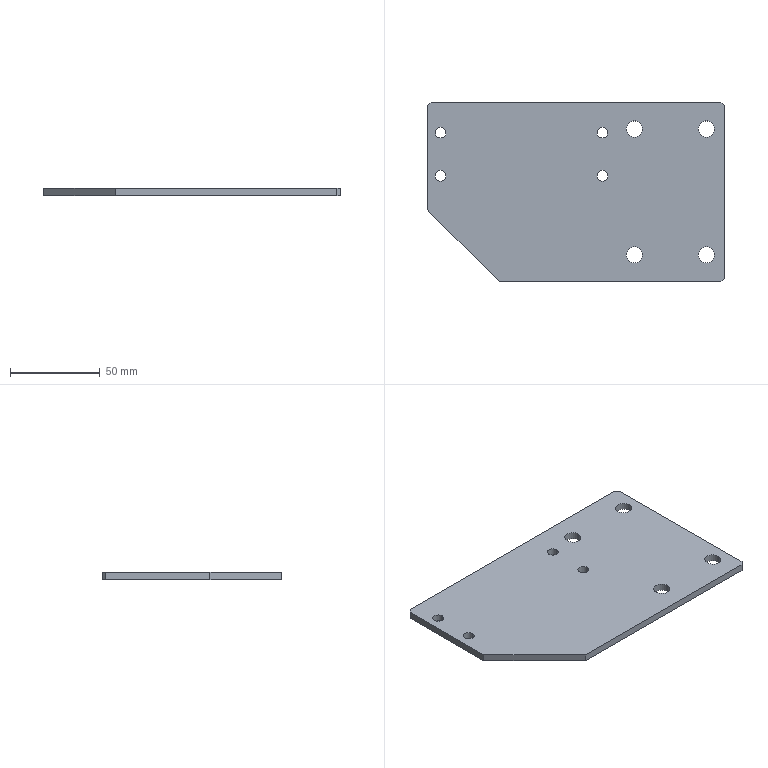Part | STEP file | Cable Carrier Bracket 1 | 1 solid | 26 faces | box 165 x 100 x 4 mm | volume 61306 mm3 | cylinder 16 | plane 10 | commonest cylinder face diameters 6 x8 9 x8